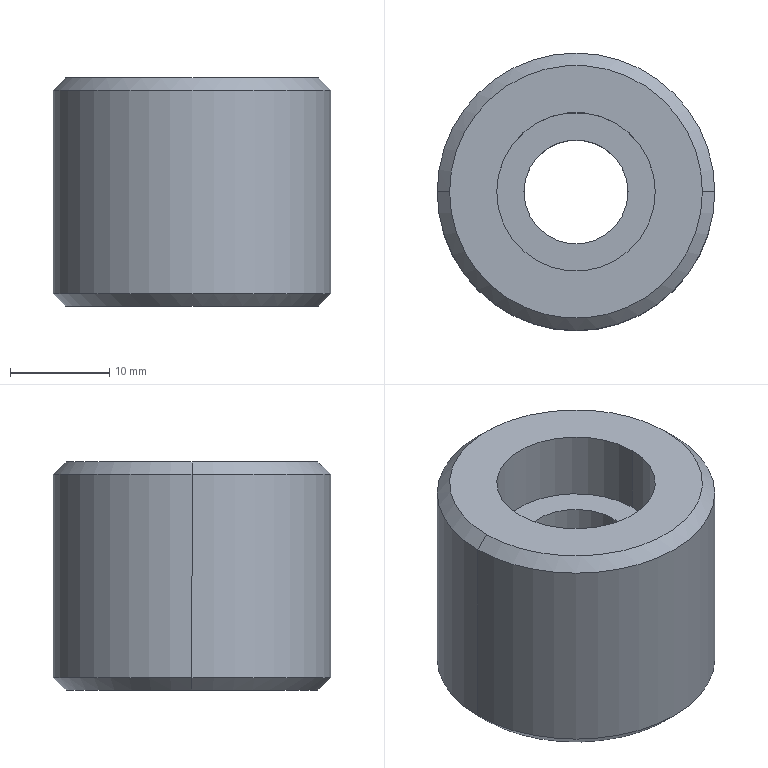Part | STEP file | IN-01-08-01-02-02 | 1 solid | 13 faces | box 28 x 28 x 23 mm | volume 11236 mm3 | cylinder 6 | cone 4 | plane 3 | commonest cylinder face diameters 10.5 x2 16 x2 28 x2
STEP:
#1=CARTESIAN_POINT('',(0.,0.,0.));
#2=DIRECTION('',(0.,0.,1.));
#3=DIRECTION('',(1.,0.,0.));
#4=AXIS2_PLACEMENT_3D('',#1,#2,#3);
#5=CARTESIAN_POINT('',(14.,0.,1.25));
#6=VERTEX_POINT('',#5);
#7=CARTESIAN_POINT('',(-14.,0.,1.25));
#8=VERTEX_POINT('',#7);
#9=CARTESIAN_POINT('',(0.,0.,1.25));
#10=DIRECTION('',(0.,0.,1.));
#11=DIRECTION('',(1.,0.,0.));
#12=AXIS2_PLACEMENT_3D('',#9,#10,#11);
#13=CIRCLE('',#12,14.);
#14=CARTESIAN_POINT('',(0.,0.,0.));
#15=DIRECTION('',(0.,0.,1.));
#16=DIRECTION('',(1.,0.,0.));
#17=AXIS2_PLACEMENT_3D('',#14,#15,#16);
#18=CYLINDRICAL_SURFACE('',#17,14.);
#19=CARTESIAN_POINT('',(0.,1.25));
#20=DIRECTION('',(1.,0.));
#21=VECTOR('',#20,1.);
#22=LINE('',#19,#21);
#23=(GEOMETRIC_REPRESENTATION_CONTEXT(2)PARAMETRIC_REPRESENTATION_CONTEXT()REPRESENTATION_CONTEXT('',''));
#24=DEFINITIONAL_REPRESENTATION('',(#22),#23);
#25=PCURVE('',#18,#24);
#26=CARTESIAN_POINT('',(0.,0.,1.25));
#27=DIRECTION('',(0.,0.,1.));
#28=DIRECTION('',(1.,0.,0.));
#29=AXIS2_PLACEMENT_3D('',#26,#27,#28);
#30=CONICAL_SURFACE('',#29,14.,0.7854);
#31=CARTESIAN_POINT('',(0.,0.));
#32=DIRECTION('',(1.,0.));
#33=VECTOR('',#32,1.);
#34=LINE('',#31,#33);
#35=(GEOMETRIC_REPRESENTATION_CONTEXT(2)PARAMETRIC_REPRESENTATION_CONTEXT()REPRESENTATION_CONTEXT('',''));
#36=DEFINITIONAL_REPRESENTATION('',(#34),#35);
#37=PCURVE('',#30,#36);
#38=SURFACE_CURVE('',#13,(#25,#37),.PCURVE_S1.);
#39=EDGE_CURVE('',#6,#8,#38,.T.);
#40=ORIENTED_EDGE('',*,*,#39,.T.);
#41=CARTESIAN_POINT('',(-14.,0.,21.75));
#42=VERTEX_POINT('',#41);
#43=CARTESIAN_POINT('',(-14.,0.,0.));
#44=DIRECTION('',(0.,0.,1.));
#45=VECTOR('',#44,1.);
#46=LINE('',#43,#45);
#47=CARTESIAN_POINT('',(3.142,0.));
#48=DIRECTION('',(0.,1.));
#49=VECTOR('',#48,1.);
#50=LINE('',#47,#49);
#51=(GEOMETRIC_REPRESENTATION_CONTEXT(2)PARAMETRIC_REPRESENTATION_CONTEXT()REPRESENTATION_CONTEXT('',''));
#52=DEFINITIONAL_REPRESENTATION('',(#50),#51);
#53=PCURVE('',#18,#52);
#54=CARTESIAN_POINT('',(0.,0.,0.));
#55=DIRECTION('',(0.,0.,1.));
#56=DIRECTION('',(1.,0.,0.));
#57=AXIS2_PLACEMENT_3D('',#54,#55,#56);
#58=CYLINDRICAL_SURFACE('',#57,14.);
#59=CARTESIAN_POINT('',(3.142,0.));
#60=DIRECTION('',(0.,1.));
#61=VECTOR('',#60,1.);
#62=LINE('',#59,#61);
#63=(GEOMETRIC_REPRESENTATION_CONTEXT(2)PARAMETRIC_REPRESENTATION_CONTEXT()REPRESENTATION_CONTEXT('',''));
#64=DEFINITIONAL_REPRESENTATION('',(#62),#63);
#65=PCURVE('',#58,#64);
#66=SURFACE_CURVE('',#46,(#53,#65),.PCURVE_S1.);
#67=EDGE_CURVE('',#8,#42,#66,.T.);
#68=ORIENTED_EDGE('',*,*,#67,.T.);
#69=CARTESIAN_POINT('',(14.,0.,21.75));
#70=VERTEX_POINT('',#69);
#71=CARTESIAN_POINT('',(0.,0.,21.75));
#72=DIRECTION('',(0.,0.,-1.));
#73=DIRECTION('',(1.,0.,0.));
#74=AXIS2_PLACEMENT_3D('',#71,#72,#73);
#75=CIRCLE('',#74,14.);
#76=CARTESIAN_POINT('',(6.283,21.75));
#77=DIRECTION('',(-1.,0.));
#78=VECTOR('',#77,1.);
#79=LINE('',#76,#78);
#80=(GEOMETRIC_REPRESENTATION_CONTEXT(2)PARAMETRIC_REPRESENTATION_CONTEXT()REPRESENTATION_CONTEXT('',''));
#81=DEFINITIONAL_REPRESENTATION('',(#79),#80);
#82=PCURVE('',#18,#81);
#83=CARTESIAN_POINT('',(0.,0.,21.75));
#84=DIRECTION('',(0.,0.,-1.));
#85=DIRECTION('',(-1.,0.,0.));
#86=AXIS2_PLACEMENT_3D('',#83,#84,#85);
#87=CONICAL_SURFACE('',#86,14.,0.7854);
#88=CARTESIAN_POINT('',(-3.142,0.));
#89=DIRECTION('',(1.,0.));
#90=VECTOR('',#89,1.);
#91=LINE('',#88,#90);
#92=(GEOMETRIC_REPRESENTATION_CONTEXT(2)PARAMETRIC_REPRESENTATION_CONTEXT()REPRESENTATION_CONTEXT('',''));
#93=DEFINITIONAL_REPRESENTATION('',(#91),#92);
#94=PCURVE('',#87,#93);
#95=SURFACE_CURVE('',#75,(#82,#94),.PCURVE_S1.);
#96=EDGE_CURVE('',#42,#70,#95,.T.);
#97=ORIENTED_EDGE('',*,*,#96,.T.);
#98=CARTESIAN_POINT('',(14.,0.,0.));
#99=DIRECTION('',(0.,0.,1.));
#100=VECTOR('',#99,1.);
#101=LINE('',#98,#100);
#102=CARTESIAN_POINT('',(0.,0.));
#103=DIRECTION('',(0.,1.));
#104=VECTOR('',#103,1.);
#105=LINE('',#102,#104);
#106=(GEOMETRIC_REPRESENTATION_CONTEXT(2)PARAMETRIC_REPRESENTATION_CONTEXT()REPRESENTATION_CONTEXT('',''));
#107=DEFINITIONAL_REPRESENTATION('',(#105),#106);
#108=PCURVE('',#18,#107);
#109=CARTESIAN_POINT('',(6.283,0.));
#110=DIRECTION('',(0.,1.));
#111=VECTOR('',#110,1.);
#112=LINE('',#109,#111);
#113=(GEOMETRIC_REPRESENTATION_CONTEXT(2)PARAMETRIC_REPRESENTATION_CONTEXT()REPRESENTATION_CONTEXT('',''));
#114=DEFINITIONAL_REPRESENTATION('',(#112),#113);
#115=PCURVE('',#58,#114);
#116=SURFACE_CURVE('',#101,(#108,#115),.PCURVE_S1.);
#117=EDGE_CURVE('',#6,#70,#116,.T.);
#118=ORIENTED_EDGE('',*,*,#117,.F.);
#119=EDGE_LOOP('',(#40,#68,#97,#118));
#120=FACE_BOUND('',#119,.T.);
#121=ADVANCED_FACE('',(#120),#18,.T.);
#122=CARTESIAN_POINT('',(12.75,0.,0.));
#123=VERTEX_POINT('',#122);
#124=CARTESIAN_POINT('',(-12.75,0.,0.));
#125=VERTEX_POINT('',#124);
#126=CARTESIAN_POINT('',(0.,0.,0.));
#127=DIRECTION('',(0.,0.,1.));
#128=DIRECTION('',(1.,0.,0.));
#129=AXIS2_PLACEMENT_3D('',#126,#127,#128);
#130=CIRCLE('',#129,12.75);
#131=CARTESIAN_POINT('',(0.,-1.25));
#132=DIRECTION('',(1.,0.));
#133=VECTOR('',#132,1.);
#134=LINE('',#131,#133);
#135=(GEOMETRIC_REPRESENTATION_CONTEXT(2)PARAMETRIC_REPRESENTATION_CONTEXT()REPRESENTATION_CONTEXT('',''));
#136=DEFINITIONAL_REPRESENTATION('',(#134),#135);
#137=PCURVE('',#30,#136);
#138=CARTESIAN_POINT('',(0.,0.,0.));
#139=DIRECTION('',(0.,0.,1.));
#140=DIRECTION('',(1.,0.,0.));
#141=AXIS2_PLACEMENT_3D('',#138,#139,#140);
#142=PLANE('',#141);
#143=CARTESIAN_POINT('',(0.,0.));
#144=DIRECTION('',(1.,0.));
#145=AXIS2_PLACEMENT_2D('',#143,#144);
#146=CIRCLE('',#145,12.75);
#147=(GEOMETRIC_REPRESENTATION_CONTEXT(2)PARAMETRIC_REPRESENTATION_CONTEXT()REPRESENTATION_CONTEXT('',''));
#148=DEFINITIONAL_REPRESENTATION('',(#146),#147);
#149=PCURVE('',#142,#148);
#150=SURFACE_CURVE('',#130,(#137,#149),.PCURVE_S1.);
#151=EDGE_CURVE('',#123,#125,#150,.T.);
#152=ORIENTED_EDGE('',*,*,#151,.T.);
#153=CARTESIAN_POINT('',(-14.,0.,1.25));
#154=DIRECTION('',(-0.7071,0.,0.7071));
#155=VECTOR('',#154,1.);
#156=LINE('',#153,#155);
#157=CARTESIAN_POINT('',(3.142,0.));
#158=DIRECTION('',(0.,1.));
#159=VECTOR('',#158,1.);
#160=LINE('',#157,#159);
#161=(GEOMETRIC_REPRESENTATION_CONTEXT(2)PARAMETRIC_REPRESENTATION_CONTEXT()REPRESENTATION_CONTEXT('',''));
#162=DEFINITIONAL_REPRESENTATION('',(#160),#161);
#163=PCURVE('',#30,#162);
#164=CARTESIAN_POINT('',(0.,0.,1.25));
#165=DIRECTION('',(0.,0.,1.));
#166=DIRECTION('',(1.,0.,0.));
#167=AXIS2_PLACEMENT_3D('',#164,#165,#166);
#168=CONICAL_SURFACE('',#167,14.,0.7854);
#169=CARTESIAN_POINT('',(3.142,0.));
#170=DIRECTION('',(0.,1.));
#171=VECTOR('',#170,1.);
#172=LINE('',#169,#171);
#173=(GEOMETRIC_REPRESENTATION_CONTEXT(2)PARAMETRIC_REPRESENTATION_CONTEXT()REPRESENTATION_CONTEXT('',''));
#174=DEFINITIONAL_REPRESENTATION('',(#172),#173);
#175=PCURVE('',#168,#174);
#176=SURFACE_CURVE('',#156,(#163,#175),.PCURVE_S1.);
#177=EDGE_CURVE('',#125,#8,#176,.T.);
#178=ORIENTED_EDGE('',*,*,#177,.T.);
#179=ORIENTED_EDGE('',*,*,#39,.F.);
#180=CARTESIAN_POINT('',(14.,0.,1.25));
#181=DIRECTION('',(0.7071,0.,0.7071));
#182=VECTOR('',#181,1.);
#183=LINE('',#180,#182);
#184=CARTESIAN_POINT('',(0.,0.));
#185=DIRECTION('',(0.,1.));
#186=VECTOR('',#185,1.);
#187=LINE('',#184,#186);
#188=(GEOMETRIC_REPRESENTATION_CONTEXT(2)PARAMETRIC_REPRESENTATION_CONTEXT()REPRESENTATION_CONTEXT('',''));
#189=DEFINITIONAL_REPRESENTATION('',(#187),#188);
#190=PCURVE('',#30,#189);
#191=CARTESIAN_POINT('',(6.283,0.));
#192=DIRECTION('',(0.,1.));
#193=VECTOR('',#192,1.);
#194=LINE('',#191,#193);
#195=(GEOMETRIC_REPRESENTATION_CONTEXT(2)PARAMETRIC_REPRESENTATION_CONTEXT()REPRESENTATION_CONTEXT('',''));
#196=DEFINITIONAL_REPRESENTATION('',(#194),#195);
#197=PCURVE('',#168,#196);
#198=SURFACE_CURVE('',#183,(#190,#197),.PCURVE_S1.);
#199=EDGE_CURVE('',#123,#6,#198,.T.);
#200=ORIENTED_EDGE('',*,*,#199,.F.);
#201=EDGE_LOOP('',(#152,#178,#179,#200));
#202=FACE_BOUND('',#201,.T.);
#203=ADVANCED_FACE('',(#202),#30,.T.);
#204=CARTESIAN_POINT('',(-12.75,0.,23.));
#205=VERTEX_POINT('',#204);
#206=CARTESIAN_POINT('',(12.75,0.,23.));
#207=VERTEX_POINT('',#206);
#208=CARTESIAN_POINT('',(0.,0.,23.));
#209=DIRECTION('',(0.,0.,-1.));
#210=DIRECTION('',(-1.,0.,0.));
#211=AXIS2_PLACEMENT_3D('',#208,#209,#210);
#212=CIRCLE('',#211,12.75);
#213=CARTESIAN_POINT('',(0.,-1.25));
#214=DIRECTION('',(1.,0.));
#215=VECTOR('',#214,1.);
#216=LINE('',#213,#215);
#217=(GEOMETRIC_REPRESENTATION_CONTEXT(2)PARAMETRIC_REPRESENTATION_CONTEXT()REPRESENTATION_CONTEXT('',''));
#218=DEFINITIONAL_REPRESENTATION('',(#216),#217);
#219=PCURVE('',#87,#218);
#220=CARTESIAN_POINT('',(0.,0.,23.));
#221=DIRECTION('',(0.,0.,1.));
#222=DIRECTION('',(1.,0.,0.));
#223=AXIS2_PLACEMENT_3D('',#220,#221,#222);
#224=PLANE('',#223);
#225=CARTESIAN_POINT('',(-12.75,0.));
#226=CARTESIAN_POINT('',(-12.75,22.084));
#227=CARTESIAN_POINT('',(6.375,11.042));
#228=CARTESIAN_POINT('',(25.5,0.));
#229=CARTESIAN_POINT('',(6.375,-11.042));
#230=CARTESIAN_POINT('',(-12.75,-22.084));
#231=CARTESIAN_POINT('',(-12.75,0.));
#232=(BOUNDED_CURVE()B_SPLINE_CURVE(2,(#225,#226,#227,#228,#229,#230,#231),.UNSPECIFIED.,.T.,.F.)B_SPLINE_CURVE_WITH_KNOTS((1,2,2,2,2,1),(-2.094,0.,2.094,4.189,6.283,8.378),.UNSPECIFIED.)CURVE()GEOMETRIC_REPRESENTATION_ITEM()RATIONAL_B_SPLINE_CURVE((1.,0.5,1.,0.5,1.,0.5,1.))REPRESENTATION_ITEM(''));
#233=(GEOMETRIC_REPRESENTATION_CONTEXT(2)PARAMETRIC_REPRESENTATION_CONTEXT()REPRESENTATION_CONTEXT('',''));
#234=DEFINITIONAL_REPRESENTATION('',(#232),#233);
#235=PCURVE('',#224,#234);
#236=SURFACE_CURVE('',#212,(#219,#235),.PCURVE_S1.);
#237=EDGE_CURVE('',#205,#207,#236,.T.);
#238=ORIENTED_EDGE('',*,*,#237,.T.);
#239=CARTESIAN_POINT('',(14.,0.,21.75));
#240=DIRECTION('',(0.7071,0.,-0.7071));
#241=VECTOR('',#240,1.);
#242=LINE('',#239,#241);
#243=CARTESIAN_POINT('',(3.142,0.));
#244=DIRECTION('',(0.,1.));
#245=VECTOR('',#244,1.);
#246=LINE('',#243,#245);
#247=(GEOMETRIC_REPRESENTATION_CONTEXT(2)PARAMETRIC_REPRESENTATION_CONTEXT()REPRESENTATION_CONTEXT('',''));
#248=DEFINITIONAL_REPRESENTATION('',(#246),#247);
#249=PCURVE('',#87,#248);
#250=CARTESIAN_POINT('',(0.,0.,21.75));
#251=DIRECTION('',(0.,0.,-1.));
#252=DIRECTION('',(-1.,0.,0.));
#253=AXIS2_PLACEMENT_3D('',#250,#251,#252);
#254=CONICAL_SURFACE('',#253,14.,0.7854);
#255=CARTESIAN_POINT('',(3.142,0.));
#256=DIRECTION('',(0.,1.));
#257=VECTOR('',#256,1.);
#258=LINE('',#255,#257);
#259=(GEOMETRIC_REPRESENTATION_CONTEXT(2)PARAMETRIC_REPRESENTATION_CONTEXT()REPRESENTATION_CONTEXT('',''));
#260=DEFINITIONAL_REPRESENTATION('',(#258),#259);
#261=PCURVE('',#254,#260);
#262=SURFACE_CURVE('',#242,(#249,#261),.PCURVE_S1.);
#263=EDGE_CURVE('',#207,#70,#262,.T.);
#264=ORIENTED_EDGE('',*,*,#263,.T.);
#265=ORIENTED_EDGE('',*,*,#96,.F.);
#266=CARTESIAN_POINT('',(-14.,0.,21.75));
#267=DIRECTION('',(-0.7071,0.,-0.7071));
#268=VECTOR('',#267,1.);
#269=LINE('',#266,#268);
#270=CARTESIAN_POINT('',(0.,0.));
#271=DIRECTION('',(0.,1.));
#272=VECTOR('',#271,1.);
#273=LINE('',#270,#272);
#274=(GEOMETRIC_REPRESENTATION_CONTEXT(2)PARAMETRIC_REPRESENTATION_CONTEXT()REPRESENTATION_CONTEXT('',''));
#275=DEFINITIONAL_REPRESENTATION('',(#273),#274);
#276=PCURVE('',#87,#275);
#277=CARTESIAN_POINT('',(6.283,0.));
#278=DIRECTION('',(0.,1.));
#279=VECTOR('',#278,1.);
#280=LINE('',#277,#279);
#281=(GEOMETRIC_REPRESENTATION_CONTEXT(2)PARAMETRIC_REPRESENTATION_CONTEXT()REPRESENTATION_CONTEXT('',''));
#282=DEFINITIONAL_REPRESENTATION('',(#280),#281);
#283=PCURVE('',#254,#282);
#284=SURFACE_CURVE('',#269,(#276,#283),.PCURVE_S1.);
#285=EDGE_CURVE('',#205,#42,#284,.T.);
#286=ORIENTED_EDGE('',*,*,#285,.F.);
#287=EDGE_LOOP('',(#238,#264,#265,#286));
#288=FACE_BOUND('',#287,.T.);
#289=ADVANCED_FACE('',(#288),#87,.T.);
#290=CARTESIAN_POINT('',(5.25,0.,0.));
#291=VERTEX_POINT('',#290);
#292=CARTESIAN_POINT('',(5.25,0.,16.));
#293=VERTEX_POINT('',#292);
#294=CARTESIAN_POINT('',(5.25,0.,0.));
#295=DIRECTION('',(0.,0.,1.));
#296=VECTOR('',#295,1.);
#297=LINE('',#294,#296);
#298=CARTESIAN_POINT('',(0.,0.,0.));
#299=DIRECTION('',(0.,0.,1.));
#300=DIRECTION('',(1.,0.,0.));
#301=AXIS2_PLACEMENT_3D('',#298,#299,#300);
#302=CYLINDRICAL_SURFACE('',#301,5.25);
#303=CARTESIAN_POINT('',(6.283,0.));
#304=DIRECTION('',(0.,1.));
#305=VECTOR('',#304,1.);
#306=LINE('',#303,#305);
#307=(GEOMETRIC_REPRESENTATION_CONTEXT(2)PARAMETRIC_REPRESENTATION_CONTEXT()REPRESENTATION_CONTEXT('',''));
#308=DEFINITIONAL_REPRESENTATION('',(#306),#307);
#309=PCURVE('',#302,#308);
#310=CARTESIAN_POINT('',(0.,0.,0.));
#311=DIRECTION('',(0.,0.,1.));
#312=DIRECTION('',(1.,0.,0.));
#313=AXIS2_PLACEMENT_3D('',#310,#311,#312);
#314=CYLINDRICAL_SURFACE('',#313,5.25);
#315=CARTESIAN_POINT('',(0.,0.));
#316=DIRECTION('',(0.,1.));
#317=VECTOR('',#316,1.);
#318=LINE('',#315,#317);
#319=(GEOMETRIC_REPRESENTATION_CONTEXT(2)PARAMETRIC_REPRESENTATION_CONTEXT()REPRESENTATION_CONTEXT('',''));
#320=DEFINITIONAL_REPRESENTATION('',(#318),#319);
#321=PCURVE('',#314,#320);
#322=SURFACE_CURVE('',#297,(#309,#321),.PCURVE_S1.);
#323=EDGE_CURVE('',#291,#293,#322,.T.);
#324=ORIENTED_EDGE('',*,*,#323,.T.);
#325=CARTESIAN_POINT('',(-5.25,0.,16.));
#326=VERTEX_POINT('',#325);
#327=CARTESIAN_POINT('',(0.,0.,16.));
#328=DIRECTION('',(0.,0.,-1.));
#329=DIRECTION('',(1.,0.,0.));
#330=AXIS2_PLACEMENT_3D('',#327,#328,#329);
#331=CIRCLE('',#330,5.25);
#332=CARTESIAN_POINT('',(6.283,16.));
#333=DIRECTION('',(-1.,0.));
#334=VECTOR('',#333,1.);
#335=LINE('',#332,#334);
#336=(GEOMETRIC_REPRESENTATION_CONTEXT(2)PARAMETRIC_REPRESENTATION_CONTEXT()REPRESENTATION_CONTEXT('',''));
#337=DEFINITIONAL_REPRESENTATION('',(#335),#336);
#338=PCURVE('',#302,#337);
#339=CARTESIAN_POINT('',(0.,0.,16.));
#340=DIRECTION('',(0.,0.,1.));
#341=DIRECTION('',(1.,0.,0.));
#342=AXIS2_PLACEMENT_3D('',#339,#340,#341);
#343=PLANE('',#342);
#344=CARTESIAN_POINT('',(5.25,0.));
#345=CARTESIAN_POINT('',(5.25,-9.093));
#346=CARTESIAN_POINT('',(-2.625,-4.547));
#347=CARTESIAN_POINT('',(-10.5,0.));
#348=CARTESIAN_POINT('',(-2.625,4.547));
#349=CARTESIAN_POINT('',(5.25,9.093));
#350=CARTESIAN_POINT('',(5.25,0.));
#351=(BOUNDED_CURVE()B_SPLINE_CURVE(2,(#344,#345,#346,#347,#348,#349,#350),.UNSPECIFIED.,.T.,.F.)B_SPLINE_CURVE_WITH_KNOTS((1,2,2,2,2,1),(-2.094,0.,2.094,4.189,6.283,8.378),.UNSPECIFIED.)CURVE()GEOMETRIC_REPRESENTATION_ITEM()RATIONAL_B_SPLINE_CURVE((1.,0.5,1.,0.5,1.,0.5,1.))REPRESENTATION_ITEM(''));
#352=(GEOMETRIC_REPRESENTATION_CONTEXT(2)PARAMETRIC_REPRESENTATION_CONTEXT()REPRESENTATION_CONTEXT('',''));
#353=DEFINITIONAL_REPRESENTATION('',(#351),#352);
#354=PCURVE('',#343,#353);
#355=SURFACE_CURVE('',#331,(#338,#354),.PCURVE_S1.);
#356=EDGE_CURVE('',#293,#326,#355,.T.);
#357=ORIENTED_EDGE('',*,*,#356,.T.);
#358=CARTESIAN_POINT('',(-5.25,0.,0.));
#359=VERTEX_POINT('',#358);
#360=CARTESIAN_POINT('',(-5.25,0.,0.));
#361=DIRECTION('',(0.,0.,1.));
#362=VECTOR('',#361,1.);
#363=LINE('',#360,#362);
#364=CARTESIAN_POINT('',(3.142,0.));
#365=DIRECTION('',(0.,1.));
#366=VECTOR('',#365,1.);
#367=LINE('',#364,#366);
#368=(GEOMETRIC_REPRESENTATION_CONTEXT(2)PARAMETRIC_REPRESENTATION_CONTEXT()REPRESENTATION_CONTEXT('',''));
#369=DEFINITIONAL_REPRESENTATION('',(#367),#368);
#370=PCURVE('',#302,#369);
#371=CARTESIAN_POINT('',(3.142,0.));
#372=DIRECTION('',(0.,1.));
#373=VECTOR('',#372,1.);
#374=LINE('',#371,#373);
#375=(GEOMETRIC_REPRESENTATION_CONTEXT(2)PARAMETRIC_REPRESENTATION_CONTEXT()REPRESENTATION_CONTEXT('',''));
#376=DEFINITIONAL_REPRESENTATION('',(#374),#375);
#377=PCURVE('',#314,#376);
#378=SURFACE_CURVE('',#363,(#370,#377),.PCURVE_S1.);
#379=EDGE_CURVE('',#359,#326,#378,.T.);
#380=ORIENTED_EDGE('',*,*,#379,.F.);
#381=CARTESIAN_POINT('',(0.,0.,0.));
#382=DIRECTION('',(0.,0.,-1.));
#383=DIRECTION('',(1.,0.,0.));
#384=AXIS2_PLACEMENT_3D('',#381,#382,#383);
#385=CIRCLE('',#384,5.25);
#386=CARTESIAN_POINT('',(6.283,0.));
#387=DIRECTION('',(-1.,0.));
#388=VECTOR('',#387,1.);
#389=LINE('',#386,#388);
#390=(GEOMETRIC_REPRESENTATION_CONTEXT(2)PARAMETRIC_REPRESENTATION_CONTEXT()REPRESENTATION_CONTEXT('',''));
#391=DEFINITIONAL_REPRESENTATION('',(#389),#390);
#392=PCURVE('',#302,#391);
#393=CARTESIAN_POINT('',(5.25,0.));
#394=CARTESIAN_POINT('',(5.25,-9.093));
#395=CARTESIAN_POINT('',(-2.625,-4.547));
#396=CARTESIAN_POINT('',(-10.5,0.));
#397=CARTESIAN_POINT('',(-2.625,4.547));
#398=CARTESIAN_POINT('',(5.25,9.093));
#399=CARTESIAN_POINT('',(5.25,0.));
#400=(BOUNDED_CURVE()B_SPLINE_CURVE(2,(#393,#394,#395,#396,#397,#398,#399),.UNSPECIFIED.,.T.,.F.)B_SPLINE_CURVE_WITH_KNOTS((1,2,2,2,2,1),(-2.094,0.,2.094,4.189,6.283,8.378),.UNSPECIFIED.)CURVE()GEOMETRIC_REPRESENTATION_ITEM()RATIONAL_B_SPLINE_CURVE((1.,0.5,1.,0.5,1.,0.5,1.))REPRESENTATION_ITEM(''));
#401=(GEOMETRIC_REPRESENTATION_CONTEXT(2)PARAMETRIC_REPRESENTATION_CONTEXT()REPRESENTATION_CONTEXT('',''));
#402=DEFINITIONAL_REPRESENTATION('',(#400),#401);
#403=PCURVE('',#142,#402);
#404=SURFACE_CURVE('',#385,(#392,#403),.PCURVE_S1.);
#405=EDGE_CURVE('',#291,#359,#404,.T.);
#406=ORIENTED_EDGE('',*,*,#405,.F.);
#407=EDGE_LOOP('',(#324,#357,#380,#406));
#408=FACE_BOUND('',#407,.F.);
#409=ADVANCED_FACE('',(#408),#302,.F.);
#410=CARTESIAN_POINT('',(-8.,0.,23.));
#411=VERTEX_POINT('',#410);
#412=CARTESIAN_POINT('',(-8.,0.,16.));
#413=VERTEX_POINT('',#412);
#414=CARTESIAN_POINT('',(-8.,0.,23.));
#415=DIRECTION('',(0.,0.,-1.));
#416=VECTOR('',#415,1.);
#417=LINE('',#414,#416);
#418=CARTESIAN_POINT('',(0.,0.,23.));
#419=DIRECTION('',(0.,0.,-1.));
#420=DIRECTION('',(-1.,0.,0.));
#421=AXIS2_PLACEMENT_3D('',#418,#419,#420);
#422=CYLINDRICAL_SURFACE('',#421,8.);
#423=CARTESIAN_POINT('',(6.283,0.));
#424=DIRECTION('',(0.,1.));
#425=VECTOR('',#424,1.);
#426=LINE('',#423,#425);
#427=(GEOMETRIC_REPRESENTATION_CONTEXT(2)PARAMETRIC_REPRESENTATION_CONTEXT()REPRESENTATION_CONTEXT('',''));
#428=DEFINITIONAL_REPRESENTATION('',(#426),#427);
#429=PCURVE('',#422,#428);
#430=CARTESIAN_POINT('',(0.,0.,23.));
#431=DIRECTION('',(0.,0.,-1.));
#432=DIRECTION('',(-1.,0.,0.));
#433=AXIS2_PLACEMENT_3D('',#430,#431,#432);
#434=CYLINDRICAL_SURFACE('',#433,8.);
#435=CARTESIAN_POINT('',(0.,0.));
#436=DIRECTION('',(0.,1.));
#437=VECTOR('',#436,1.);
#438=LINE('',#435,#437);
#439=(GEOMETRIC_REPRESENTATION_CONTEXT(2)PARAMETRIC_REPRESENTATION_CONTEXT()REPRESENTATION_CONTEXT('',''));
#440=DEFINITIONAL_REPRESENTATION('',(#438),#439);
#441=PCURVE('',#434,#440);
#442=SURFACE_CURVE('',#417,(#429,#441),.PCURVE_S1.);
#443=EDGE_CURVE('',#411,#413,#442,.T.);
#444=ORIENTED_EDGE('',*,*,#443,.T.);
#445=CARTESIAN_POINT('',(8.,0.,16.));
#446=VERTEX_POINT('',#445);
#447=CARTESIAN_POINT('',(0.,0.,16.));
#448=DIRECTION('',(0.,0.,1.));
#449=DIRECTION('',(-1.,0.,0.));
#450=AXIS2_PLACEMENT_3D('',#447,#448,#449);
#451=CIRCLE('',#450,8.);
#452=CARTESIAN_POINT('',(6.283,7.));
#453=DIRECTION('',(-1.,0.));
#454=VECTOR('',#453,1.);
#455=LINE('',#452,#454);
#456=(GEOMETRIC_REPRESENTATION_CONTEXT(2)PARAMETRIC_REPRESENTATION_CONTEXT()REPRESENTATION_CONTEXT('',''));
#457=DEFINITIONAL_REPRESENTATION('',(#455),#456);
#458=PCURVE('',#422,#457);
#459=CARTESIAN_POINT('',(0.,0.));
#460=DIRECTION('',(-1.,0.));
#461=AXIS2_PLACEMENT_2D('',#459,#460);
#462=CIRCLE('',#461,8.);
#463=(GEOMETRIC_REPRESENTATION_CONTEXT(2)PARAMETRIC_REPRESENTATION_CONTEXT()REPRESENTATION_CONTEXT('',''));
#464=DEFINITIONAL_REPRESENTATION('',(#462),#463);
#465=PCURVE('',#343,#464);
#466=SURFACE_CURVE('',#451,(#458,#465),.PCURVE_S1.);
#467=EDGE_CURVE('',#413,#446,#466,.T.);
#468=ORIENTED_EDGE('',*,*,#467,.T.);
#469=CARTESIAN_POINT('',(8.,0.,23.));
#470=VERTEX_POINT('',#469);
#471=CARTESIAN_POINT('',(8.,0.,23.));
#472=DIRECTION('',(0.,0.,-1.));
#473=VECTOR('',#472,1.);
#474=LINE('',#471,#473);
#475=CARTESIAN_POINT('',(3.142,0.));
#476=DIRECTION('',(0.,1.));
#477=VECTOR('',#476,1.);
#478=LINE('',#475,#477);
#479=(GEOMETRIC_REPRESENTATION_CONTEXT(2)PARAMETRIC_REPRESENTATION_CONTEXT()REPRESENTATION_CONTEXT('',''));
#480=DEFINITIONAL_REPRESENTATION('',(#478),#479);
#481=PCURVE('',#422,#480);
#482=CARTESIAN_POINT('',(3.142,0.));
#483=DIRECTION('',(0.,1.));
#484=VECTOR('',#483,1.);
#485=LINE('',#482,#484);
#486=(GEOMETRIC_REPRESENTATION_CONTEXT(2)PARAMETRIC_REPRESENTATION_CONTEXT()REPRESENTATION_CONTEXT('',''));
#487=DEFINITIONAL_REPRESENTATION('',(#485),#486);
#488=PCURVE('',#434,#487);
#489=SURFACE_CURVE('',#474,(#481,#488),.PCURVE_S1.);
#490=EDGE_CURVE('',#470,#446,#489,.T.);
#491=ORIENTED_EDGE('',*,*,#490,.F.);
#492=CARTESIAN_POINT('',(0.,0.,23.));
#493=DIRECTION('',(0.,0.,-1.));
#494=DIRECTION('',(-1.,0.,0.));
#495=AXIS2_PLACEMENT_3D('',#492,#493,#494);
#496=CIRCLE('',#495,8.);
#497=CARTESIAN_POINT('',(0.,0.));
#498=DIRECTION('',(1.,0.));
#499=VECTOR('',#498,1.);
#500=LINE('',#497,#499);
#501=(GEOMETRIC_REPRESENTATION_CONTEXT(2)PARAMETRIC_REPRESENTATION_CONTEXT()REPRESENTATION_CONTEXT('',''));
#502=DEFINITIONAL_REPRESENTATION('',(#500),#501);
#503=PCURVE('',#422,#502);
#504=CARTESIAN_POINT('',(-8.,0.));
#505=CARTESIAN_POINT('',(-8.,13.856));
#506=CARTESIAN_POINT('',(4.,6.928));
#507=CARTESIAN_POINT('',(16.,0.));
#508=CARTESIAN_POINT('',(4.,-6.928));
#509=CARTESIAN_POINT('',(-8.,-13.856));
#510=CARTESIAN_POINT('',(-8.,0.));
#511=(BOUNDED_CURVE()B_SPLINE_CURVE(2,(#504,#505,#506,#507,#508,#509,#510),.UNSPECIFIED.,.T.,.F.)B_SPLINE_CURVE_WITH_KNOTS((1,2,2,2,2,1),(-2.094,0.,2.094,4.189,6.283,8.378),.UNSPECIFIED.)CURVE()GEOMETRIC_REPRESENTATION_ITEM()RATIONAL_B_SPLINE_CURVE((1.,0.5,1.,0.5,1.,0.5,1.))REPRESENTATION_ITEM(''));
#512=(GEOMETRIC_REPRESENTATION_CONTEXT(2)PARAMETRIC_REPRESENTATION_CONTEXT()REPRESENTATION_CONTEXT('',''));
#513=DEFINITIONAL_REPRESENTATION('',(#511),#512);
#514=PCURVE('',#224,#513);
#515=SURFACE_CURVE('',#496,(#503,#514),.PCURVE_S1.);
#516=EDGE_CURVE('',#470,#411,#515,.T.);
#517=ORIENTED_EDGE('',*,*,#516,.T.);
#518=EDGE_LOOP('',(#444,#468,#491,#517));
#519=FACE_BOUND('',#518,.F.);
#520=ADVANCED_FACE('',(#519),#422,.F.);
#521=ORIENTED_EDGE('',*,*,#67,.F.);
#522=CARTESIAN_POINT('',(0.,0.,1.25));
#523=DIRECTION('',(0.,0.,1.));
#524=DIRECTION('',(1.,0.,0.));
#525=AXIS2_PLACEMENT_3D('',#522,#523,#524);
#526=CIRCLE('',#525,14.);
#527=CARTESIAN_POINT('',(0.,1.25));
#528=DIRECTION('',(1.,0.));
#529=VECTOR('',#528,1.);
#530=LINE('',#527,#529);
#531=(GEOMETRIC_REPRESENTATION_CONTEXT(2)PARAMETRIC_REPRESENTATION_CONTEXT()REPRESENTATION_CONTEXT('',''));
#532=DEFINITIONAL_REPRESENTATION('',(#530),#531);
#533=PCURVE('',#58,#532);
#534=CARTESIAN_POINT('',(0.,0.));
#535=DIRECTION('',(1.,0.));
#536=VECTOR('',#535,1.);
#537=LINE('',#534,#536);
#538=(GEOMETRIC_REPRESENTATION_CONTEXT(2)PARAMETRIC_REPRESENTATION_CONTEXT()REPRESENTATION_CONTEXT('',''));
#539=DEFINITIONAL_REPRESENTATION('',(#537),#538);
#540=PCURVE('',#168,#539);
#541=SURFACE_CURVE('',#526,(#533,#540),.PCURVE_S1.);
#542=EDGE_CURVE('',#8,#6,#541,.T.);
#543=ORIENTED_EDGE('',*,*,#542,.T.);
#544=ORIENTED_EDGE('',*,*,#117,.T.);
#545=CARTESIAN_POINT('',(0.,0.,21.75));
#546=DIRECTION('',(0.,0.,-1.));
#547=DIRECTION('',(1.,0.,0.));
#548=AXIS2_PLACEMENT_3D('',#545,#546,#547);
#549=CIRCLE('',#548,14.);
#550=CARTESIAN_POINT('',(6.283,21.75));
#551=DIRECTION('',(-1.,0.));
#552=VECTOR('',#551,1.);
#553=LINE('',#550,#552);
#554=(GEOMETRIC_REPRESENTATION_CONTEXT(2)PARAMETRIC_REPRESENTATION_CONTEXT()REPRESENTATION_CONTEXT('',''));
#555=DEFINITIONAL_REPRESENTATION('',(#553),#554);
#556=PCURVE('',#58,#555);
#557=CARTESIAN_POINT('',(3.142,0.));
#558=DIRECTION('',(1.,0.));
#559=VECTOR('',#558,1.);
#560=LINE('',#557,#559);
#561=(GEOMETRIC_REPRESENTATION_CONTEXT(2)PARAMETRIC_REPRESENTATION_CONTEXT()REPRESENTATION_CONTEXT('',''));
#562=DEFINITIONAL_REPRESENTATION('',(#560),#561);
#563=PCURVE('',#254,#562);
#564=SURFACE_CURVE('',#549,(#556,#563),.PCURVE_S1.);
#565=EDGE_CURVE('',#70,#42,#564,.T.);
#566=ORIENTED_EDGE('',*,*,#565,.T.);
#567=EDGE_LOOP('',(#521,#543,#544,#566));
#568=FACE_BOUND('',#567,.T.);
#569=ADVANCED_FACE('',(#568),#58,.T.);
#570=ORIENTED_EDGE('',*,*,#177,.F.);
#571=CARTESIAN_POINT('',(0.,0.,0.));
#572=DIRECTION('',(0.,0.,1.));
#573=DIRECTION('',(1.,0.,0.));
#574=AXIS2_PLACEMENT_3D('',#571,#572,#573);
#575=CIRCLE('',#574,12.75);
#576=CARTESIAN_POINT('',(0.,-1.25));
#577=DIRECTION('',(1.,0.));
#578=VECTOR('',#577,1.);
#579=LINE('',#576,#578);
#580=(GEOMETRIC_REPRESENTATION_CONTEXT(2)PARAMETRIC_REPRESENTATION_CONTEXT()REPRESENTATION_CONTEXT('',''));
#581=DEFINITIONAL_REPRESENTATION('',(#579),#580);
#582=PCURVE('',#168,#581);
#583=CARTESIAN_POINT('',(0.,0.));
#584=DIRECTION('',(1.,0.));
#585=AXIS2_PLACEMENT_2D('',#583,#584);
#586=CIRCLE('',#585,12.75);
#587=(GEOMETRIC_REPRESENTATION_CONTEXT(2)PARAMETRIC_REPRESENTATION_CONTEXT()REPRESENTATION_CONTEXT('',''));
#588=DEFINITIONAL_REPRESENTATION('',(#586),#587);
#589=PCURVE('',#142,#588);
#590=SURFACE_CURVE('',#575,(#582,#589),.PCURVE_S1.);
#591=EDGE_CURVE('',#125,#123,#590,.T.);
#592=ORIENTED_EDGE('',*,*,#591,.T.);
#593=ORIENTED_EDGE('',*,*,#199,.T.);
#594=ORIENTED_EDGE('',*,*,#542,.F.);
#595=EDGE_LOOP('',(#570,#592,#593,#594));
#596=FACE_BOUND('',#595,.T.);
#597=ADVANCED_FACE('',(#596),#168,.T.);
#598=ORIENTED_EDGE('',*,*,#263,.F.);
#599=CARTESIAN_POINT('',(0.,0.,23.));
#600=DIRECTION('',(0.,0.,-1.));
#601=DIRECTION('',(-1.,0.,0.));
#602=AXIS2_PLACEMENT_3D('',#599,#600,#601);
#603=CIRCLE('',#602,12.75);
#604=CARTESIAN_POINT('',(0.,-1.25));
#605=DIRECTION('',(1.,0.));
#606=VECTOR('',#605,1.);
#607=LINE('',#604,#606);
#608=(GEOMETRIC_REPRESENTATION_CONTEXT(2)PARAMETRIC_REPRESENTATION_CONTEXT()REPRESENTATION_CONTEXT('',''));
#609=DEFINITIONAL_REPRESENTATION('',(#607),#608);
#610=PCURVE('',#254,#609);
#611=CARTESIAN_POINT('',(-12.75,0.));
#612=CARTESIAN_POINT('',(-12.75,22.084));
#613=CARTESIAN_POINT('',(6.375,11.042));
#614=CARTESIAN_POINT('',(25.5,0.));
#615=CARTESIAN_POINT('',(6.375,-11.042));
#616=CARTESIAN_POINT('',(-12.75,-22.084));
#617=CARTESIAN_POINT('',(-12.75,0.));
#618=(BOUNDED_CURVE()B_SPLINE_CURVE(2,(#611,#612,#613,#614,#615,#616,#617),.UNSPECIFIED.,.T.,.F.)B_SPLINE_CURVE_WITH_KNOTS((1,2,2,2,2,1),(-2.094,0.,2.094,4.189,6.283,8.378),.UNSPECIFIED.)CURVE()GEOMETRIC_REPRESENTATION_ITEM()RATIONAL_B_SPLINE_CURVE((1.,0.5,1.,0.5,1.,0.5,1.))REPRESENTATION_ITEM(''));
#619=(GEOMETRIC_REPRESENTATION_CONTEXT(2)PARAMETRIC_REPRESENTATION_CONTEXT()REPRESENTATION_CONTEXT('',''));
#620=DEFINITIONAL_REPRESENTATION('',(#618),#619);
#621=PCURVE('',#224,#620);
#622=SURFACE_CURVE('',#603,(#610,#621),.PCURVE_S1.);
#623=EDGE_CURVE('',#207,#205,#622,.T.);
#624=ORIENTED_EDGE('',*,*,#623,.T.);
#625=ORIENTED_EDGE('',*,*,#285,.T.);
#626=ORIENTED_EDGE('',*,*,#565,.F.);
#627=EDGE_LOOP('',(#598,#624,#625,#626));
#628=FACE_BOUND('',#627,.T.);
#629=ADVANCED_FACE('',(#628),#254,.T.);
#630=ORIENTED_EDGE('',*,*,#405,.F.);
#631=CARTESIAN_POINT('',(0.,0.,0.));
#632=DIRECTION('',(0.,0.,-1.));
#633=DIRECTION('',(1.,0.,0.));
#634=AXIS2_PLACEMENT_3D('',#631,#632,#633);
#635=CIRCLE('',#634,5.25);
#636=CARTESIAN_POINT('',(5.25,0.));
#637=CARTESIAN_POINT('',(5.25,-9.093));
#638=CARTESIAN_POINT('',(-2.625,-4.547));
#639=CARTESIAN_POINT('',(-10.5,0.));
#640=CARTESIAN_POINT('',(-2.625,4.547));
#641=CARTESIAN_POINT('',(5.25,9.093));
#642=CARTESIAN_POINT('',(5.25,0.));
#643=(BOUNDED_CURVE()B_SPLINE_CURVE(2,(#636,#637,#638,#639,#640,#641,#642),.UNSPECIFIED.,.T.,.F.)B_SPLINE_CURVE_WITH_KNOTS((1,2,2,2,2,1),(-2.094,0.,2.094,4.189,6.283,8.378),.UNSPECIFIED.)CURVE()GEOMETRIC_REPRESENTATION_ITEM()RATIONAL_B_SPLINE_CURVE((1.,0.5,1.,0.5,1.,0.5,1.))REPRESENTATION_ITEM(''));
#644=(GEOMETRIC_REPRESENTATION_CONTEXT(2)PARAMETRIC_REPRESENTATION_CONTEXT()REPRESENTATION_CONTEXT('',''));
#645=DEFINITIONAL_REPRESENTATION('',(#643),#644);
#646=PCURVE('',#142,#645);
#647=CARTESIAN_POINT('',(6.283,0.));
#648=DIRECTION('',(-1.,0.));
#649=VECTOR('',#648,1.);
#650=LINE('',#647,#649);
#651=(GEOMETRIC_REPRESENTATION_CONTEXT(2)PARAMETRIC_REPRESENTATION_CONTEXT()REPRESENTATION_CONTEXT('',''));
#652=DEFINITIONAL_REPRESENTATION('',(#650),#651);
#653=PCURVE('',#314,#652);
#654=SURFACE_CURVE('',#635,(#646,#653),.PCURVE_S1.);
#655=EDGE_CURVE('',#359,#291,#654,.T.);
#656=ORIENTED_EDGE('',*,*,#655,.F.);
#657=EDGE_LOOP('',(#630,#656));
#658=FACE_BOUND('',#657,.T.);
#659=ORIENTED_EDGE('',*,*,#151,.F.);
#660=ORIENTED_EDGE('',*,*,#591,.F.);
#661=EDGE_LOOP('',(#659,#660));
#662=FACE_BOUND('',#661,.T.);
#663=ADVANCED_FACE('',(#658,#662),#142,.F.);
#664=CARTESIAN_POINT('',(0.,0.,23.));
#665=DIRECTION('',(0.,0.,-1.));
#666=DIRECTION('',(-1.,0.,0.));
#667=AXIS2_PLACEMENT_3D('',#664,#665,#666);
#668=CIRCLE('',#667,8.);
#669=CARTESIAN_POINT('',(-8.,0.));
#670=CARTESIAN_POINT('',(-8.,13.856));
#671=CARTESIAN_POINT('',(4.,6.928));
#672=CARTESIAN_POINT('',(16.,0.));
#673=CARTESIAN_POINT('',(4.,-6.928));
#674=CARTESIAN_POINT('',(-8.,-13.856));
#675=CARTESIAN_POINT('',(-8.,0.));
#676=(BOUNDED_CURVE()B_SPLINE_CURVE(2,(#669,#670,#671,#672,#673,#674,#675),.UNSPECIFIED.,.T.,.F.)B_SPLINE_CURVE_WITH_KNOTS((1,2,2,2,2,1),(-2.094,0.,2.094,4.189,6.283,8.378),.UNSPECIFIED.)CURVE()GEOMETRIC_REPRESENTATION_ITEM()RATIONAL_B_SPLINE_CURVE((1.,0.5,1.,0.5,1.,0.5,1.))REPRESENTATION_ITEM(''));
#677=(GEOMETRIC_REPRESENTATION_CONTEXT(2)PARAMETRIC_REPRESENTATION_CONTEXT()REPRESENTATION_CONTEXT('',''));
#678=DEFINITIONAL_REPRESENTATION('',(#676),#677);
#679=PCURVE('',#224,#678);
#680=CARTESIAN_POINT('',(0.,0.));
#681=DIRECTION('',(1.,0.));
#682=VECTOR('',#681,1.);
#683=LINE('',#680,#682);
#684=(GEOMETRIC_REPRESENTATION_CONTEXT(2)PARAMETRIC_REPRESENTATION_CONTEXT()REPRESENTATION_CONTEXT('',''));
#685=DEFINITIONAL_REPRESENTATION('',(#683),#684);
#686=PCURVE('',#434,#685);
#687=SURFACE_CURVE('',#668,(#679,#686),.PCURVE_S1.);
#688=EDGE_CURVE('',#411,#470,#687,.T.);
#689=ORIENTED_EDGE('',*,*,#688,.T.);
#690=ORIENTED_EDGE('',*,*,#516,.T.);
#691=EDGE_LOOP('',(#689,#690));
#692=FACE_BOUND('',#691,.T.);
#693=ORIENTED_EDGE('',*,*,#237,.F.);
#694=ORIENTED_EDGE('',*,*,#623,.F.);
#695=EDGE_LOOP('',(#693,#694));
#696=FACE_BOUND('',#695,.T.);
#697=ADVANCED_FACE('',(#692,#696),#224,.T.);
#698=CARTESIAN_POINT('',(0.,0.,16.));
#699=DIRECTION('',(0.,0.,-1.));
#700=DIRECTION('',(1.,0.,0.));
#701=AXIS2_PLACEMENT_3D('',#698,#699,#700);
#702=CIRCLE('',#701,5.25);
#703=CARTESIAN_POINT('',(6.283,16.));
#704=DIRECTION('',(-1.,0.));
#705=VECTOR('',#704,1.);
#706=LINE('',#703,#705);
#707=(GEOMETRIC_REPRESENTATION_CONTEXT(2)PARAMETRIC_REPRESENTATION_CONTEXT()REPRESENTATION_CONTEXT('',''));
#708=DEFINITIONAL_REPRESENTATION('',(#706),#707);
#709=PCURVE('',#314,#708);
#710=CARTESIAN_POINT('',(5.25,0.));
#711=CARTESIAN_POINT('',(5.25,-9.093));
#712=CARTESIAN_POINT('',(-2.625,-4.547));
#713=CARTESIAN_POINT('',(-10.5,0.));
#714=CARTESIAN_POINT('',(-2.625,4.547));
#715=CARTESIAN_POINT('',(5.25,9.093));
#716=CARTESIAN_POINT('',(5.25,0.));
#717=(BOUNDED_CURVE()B_SPLINE_CURVE(2,(#710,#711,#712,#713,#714,#715,#716),.UNSPECIFIED.,.T.,.F.)B_SPLINE_CURVE_WITH_KNOTS((1,2,2,2,2,1),(-2.094,0.,2.094,4.189,6.283,8.378),.UNSPECIFIED.)CURVE()GEOMETRIC_REPRESENTATION_ITEM()RATIONAL_B_SPLINE_CURVE((1.,0.5,1.,0.5,1.,0.5,1.))REPRESENTATION_ITEM(''));
#718=(GEOMETRIC_REPRESENTATION_CONTEXT(2)PARAMETRIC_REPRESENTATION_CONTEXT()REPRESENTATION_CONTEXT('',''));
#719=DEFINITIONAL_REPRESENTATION('',(#717),#718);
#720=PCURVE('',#343,#719);
#721=SURFACE_CURVE('',#702,(#709,#720),.PCURVE_S1.);
#722=EDGE_CURVE('',#326,#293,#721,.T.);
#723=ORIENTED_EDGE('',*,*,#722,.T.);
#724=ORIENTED_EDGE('',*,*,#323,.F.);
#725=ORIENTED_EDGE('',*,*,#655,.F.);
#726=ORIENTED_EDGE('',*,*,#379,.T.);
#727=EDGE_LOOP('',(#723,#724,#725,#726));
#728=FACE_BOUND('',#727,.F.);
#729=ADVANCED_FACE('',(#728),#314,.F.);
#730=CARTESIAN_POINT('',(0.,0.,16.));
#731=DIRECTION('',(0.,0.,1.));
#732=DIRECTION('',(-1.,0.,0.));
#733=AXIS2_PLACEMENT_3D('',#730,#731,#732);
#734=CIRCLE('',#733,8.);
#735=CARTESIAN_POINT('',(6.283,7.));
#736=DIRECTION('',(-1.,0.));
#737=VECTOR('',#736,1.);
#738=LINE('',#735,#737);
#739=(GEOMETRIC_REPRESENTATION_CONTEXT(2)PARAMETRIC_REPRESENTATION_CONTEXT()REPRESENTATION_CONTEXT('',''));
#740=DEFINITIONAL_REPRESENTATION('',(#738),#739);
#741=PCURVE('',#434,#740);
#742=CARTESIAN_POINT('',(0.,0.));
#743=DIRECTION('',(-1.,0.));
#744=AXIS2_PLACEMENT_2D('',#742,#743);
#745=CIRCLE('',#744,8.);
#746=(GEOMETRIC_REPRESENTATION_CONTEXT(2)PARAMETRIC_REPRESENTATION_CONTEXT()REPRESENTATION_CONTEXT('',''));
#747=DEFINITIONAL_REPRESENTATION('',(#745),#746);
#748=PCURVE('',#343,#747);
#749=SURFACE_CURVE('',#734,(#741,#748),.PCURVE_S1.);
#750=EDGE_CURVE('',#446,#413,#749,.T.);
#751=ORIENTED_EDGE('',*,*,#750,.T.);
#752=ORIENTED_EDGE('',*,*,#443,.F.);
#753=ORIENTED_EDGE('',*,*,#688,.T.);
#754=ORIENTED_EDGE('',*,*,#490,.T.);
#755=EDGE_LOOP('',(#751,#752,#753,#754));
#756=FACE_BOUND('',#755,.F.);
#757=ADVANCED_FACE('',(#756),#434,.F.);
#758=ORIENTED_EDGE('',*,*,#356,.T.);
#759=ORIENTED_EDGE('',*,*,#722,.T.);
#760=EDGE_LOOP('',(#758,#759));
#761=FACE_BOUND('',#760,.T.);
#762=ORIENTED_EDGE('',*,*,#467,.T.);
#763=ORIENTED_EDGE('',*,*,#750,.T.);
#764=EDGE_LOOP('',(#762,#763));
#765=FACE_BOUND('',#764,.T.);
#766=ADVANCED_FACE('',(#761,#765),#343,.T.);
#767=CLOSED_SHELL('',(#121,#203,#289,#409,#520,#569,#597,#629,#663,#697,#729,#757,#766));
#768=MANIFOLD_SOLID_BREP('',#767);
#769=(LENGTH_UNIT()NAMED_UNIT(*)SI_UNIT(.MILLI.,.METRE.));
#770=UNCERTAINTY_MEASURE_WITH_UNIT(LENGTH_MEASURE(0.0000001),#769,'','');
#771=(NAMED_UNIT(*)PLANE_ANGLE_UNIT()SI_UNIT($,.RADIAN.));
#772=(NAMED_UNIT(*)SI_UNIT($,.STERADIAN.)SOLID_ANGLE_UNIT());
#773=(GEOMETRIC_REPRESENTATION_CONTEXT(3)GLOBAL_UNCERTAINTY_ASSIGNED_CONTEXT((#770))GLOBAL_UNIT_ASSIGNED_CONTEXT((#769,#771,#772))REPRESENTATION_CONTEXT('',''));
#774=ADVANCED_BREP_SHAPE_REPRESENTATION('',(#4,#768),#773);